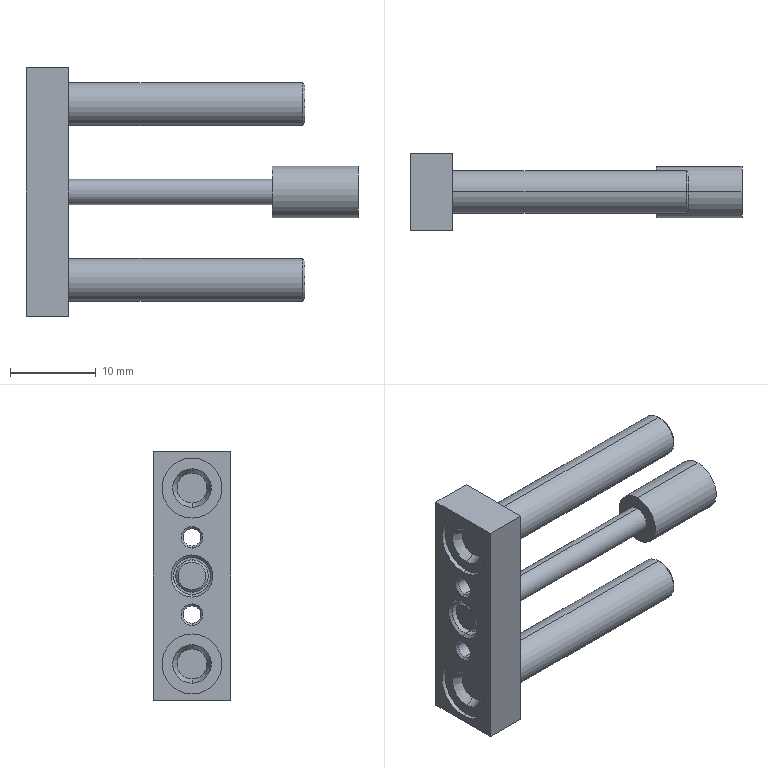Part | SolidWorks | features BaseBody 1 | 1 solid | 52 faces | box 38.7 x 9 x 29 mm | volume 2721 mm3 | cylinder 20 | cone 16 | plane 16 | commonest cylinder face diameters 2.013 x4 5 x4 7 x4 3 x2 3.8 x2 4.3 x2
STEP:
#1=CARTESIAN_POINT('',(0.2435,0.,-5.507));
#2=VERTEX_POINT('',#1);
#3=CARTESIAN_POINT('',(0.2435,0.,-3.494));
#4=VERTEX_POINT('',#3);
#5=CARTESIAN_POINT('',(0.2435,0.,-4.5));
#6=DIRECTION('',(1.,0.,0.));
#7=DIRECTION('',(0.,0.,1.));
#8=AXIS2_PLACEMENT_3D('',#5,#6,#7);
#9=CIRCLE('',#8,1.006);
#10=EDGE_CURVE('',#2,#4,#9,.T.);
#11=ORIENTED_EDGE('',*,*,#10,.F.);
#12=CARTESIAN_POINT('',(5.,0.,-5.507));
#13=VERTEX_POINT('',#12);
#14=CARTESIAN_POINT('',(5.,0.,-5.507));
#15=DIRECTION('',(1.,0.,0.));
#16=VECTOR('',#15,1000.);
#17=LINE('',#14,#16);
#18=EDGE_CURVE('',#2,#13,#17,.T.);
#19=ORIENTED_EDGE('',*,*,#18,.T.);
#20=CARTESIAN_POINT('',(5.,0.,-3.494));
#21=VERTEX_POINT('',#20);
#22=CARTESIAN_POINT('',(5.,0.,-4.5));
#23=DIRECTION('',(1.,0.,0.));
#24=DIRECTION('',(0.,0.,-1.));
#25=AXIS2_PLACEMENT_3D('',#22,#23,#24);
#26=CIRCLE('',#25,1.007);
#27=EDGE_CURVE('',#13,#21,#26,.T.);
#28=ORIENTED_EDGE('',*,*,#27,.T.);
#29=CARTESIAN_POINT('',(5.,0.,-3.494));
#30=DIRECTION('',(1.,0.,0.));
#31=VECTOR('',#30,1000.);
#32=LINE('',#29,#31);
#33=EDGE_CURVE('',#4,#21,#32,.T.);
#34=ORIENTED_EDGE('',*,*,#33,.F.);
#35=EDGE_LOOP('',(#11,#19,#28,#34));
#36=FACE_OUTER_BOUND('',#35,.T.);
#37=CARTESIAN_POINT('',(5.,0.,-4.5));
#38=DIRECTION('',(1.,0.,0.));
#39=DIRECTION('',(0.,0.,1.));
#40=AXIS2_PLACEMENT_3D('',#37,#38,#39);
#41=CYLINDRICAL_SURFACE('',#40,1.006);
#42=ADVANCED_FACE('',(#36),#41,.F.);
#43=ORIENTED_EDGE('',*,*,#10,.T.);
#44=CARTESIAN_POINT('',(0.,0.,-3.25));
#45=VERTEX_POINT('',#44);
#46=CARTESIAN_POINT('',(0.,0.,-3.25));
#47=DIRECTION('',(-0.7071,0.,0.7071));
#48=VECTOR('',#47,1000.);
#49=LINE('',#46,#48);
#50=EDGE_CURVE('',#4,#45,#49,.T.);
#51=ORIENTED_EDGE('',*,*,#50,.T.);
#52=CARTESIAN_POINT('',(0.,0.,-5.75));
#53=VERTEX_POINT('',#52);
#54=CARTESIAN_POINT('',(0.,0.,-4.5));
#55=DIRECTION('',(1.,0.,0.));
#56=DIRECTION('',(0.,-0.000000142,1.));
#57=AXIS2_PLACEMENT_3D('',#54,#55,#56);
#58=CIRCLE('',#57,1.25);
#59=EDGE_CURVE('',#53,#45,#58,.T.);
#60=ORIENTED_EDGE('',*,*,#59,.F.);
#61=CARTESIAN_POINT('',(0.,0.,-5.75));
#62=DIRECTION('',(-0.7071,0.,-0.7071));
#63=VECTOR('',#62,1000.);
#64=LINE('',#61,#63);
#65=EDGE_CURVE('',#2,#53,#64,.T.);
#66=ORIENTED_EDGE('',*,*,#65,.F.);
#67=EDGE_LOOP('',(#43,#51,#60,#66));
#68=FACE_OUTER_BOUND('',#67,.T.);
#69=CARTESIAN_POINT('',(0.,0.,-4.5));
#70=DIRECTION('',(-1.,0.,0.));
#71=DIRECTION('',(0.,0.,-1.));
#72=AXIS2_PLACEMENT_3D('',#69,#70,#71);
#73=CONICAL_SURFACE('',#72,1.25,0.7854);
#74=ADVANCED_FACE('',(#68),#73,.F.);
#75=CARTESIAN_POINT('',(0.2435,0.,3.494));
#76=VERTEX_POINT('',#75);
#77=CARTESIAN_POINT('',(0.2435,0.,5.507));
#78=VERTEX_POINT('',#77);
#79=CARTESIAN_POINT('',(0.2435,0.,4.5));
#80=DIRECTION('',(1.,0.,0.));
#81=DIRECTION('',(0.,0.,1.));
#82=AXIS2_PLACEMENT_3D('',#79,#80,#81);
#83=CIRCLE('',#82,1.007);
#84=EDGE_CURVE('',#76,#78,#83,.T.);
#85=ORIENTED_EDGE('',*,*,#84,.F.);
#86=CARTESIAN_POINT('',(5.,0.,3.494));
#87=VERTEX_POINT('',#86);
#88=CARTESIAN_POINT('',(5.,0.,3.494));
#89=DIRECTION('',(1.,0.,0.));
#90=VECTOR('',#89,1000.);
#91=LINE('',#88,#90);
#92=EDGE_CURVE('',#76,#87,#91,.T.);
#93=ORIENTED_EDGE('',*,*,#92,.T.);
#94=CARTESIAN_POINT('',(5.,0.,5.507));
#95=VERTEX_POINT('',#94);
#96=CARTESIAN_POINT('',(5.,0.,4.5));
#97=DIRECTION('',(1.,0.,0.));
#98=DIRECTION('',(0.,0.,-1.));
#99=AXIS2_PLACEMENT_3D('',#96,#97,#98);
#100=CIRCLE('',#99,1.006);
#101=EDGE_CURVE('',#87,#95,#100,.T.);
#102=ORIENTED_EDGE('',*,*,#101,.T.);
#103=CARTESIAN_POINT('',(5.,0.,5.507));
#104=DIRECTION('',(1.,0.,0.));
#105=VECTOR('',#104,1000.);
#106=LINE('',#103,#105);
#107=EDGE_CURVE('',#78,#95,#106,.T.);
#108=ORIENTED_EDGE('',*,*,#107,.F.);
#109=EDGE_LOOP('',(#85,#93,#102,#108));
#110=FACE_OUTER_BOUND('',#109,.T.);
#111=CARTESIAN_POINT('',(5.,0.,4.5));
#112=DIRECTION('',(1.,0.,0.));
#113=DIRECTION('',(0.,0.,1.));
#114=AXIS2_PLACEMENT_3D('',#111,#112,#113);
#115=CYLINDRICAL_SURFACE('',#114,1.007);
#116=ADVANCED_FACE('',(#110),#115,.F.);
#117=ORIENTED_EDGE('',*,*,#84,.T.);
#118=CARTESIAN_POINT('',(0.,0.,5.75));
#119=VERTEX_POINT('',#118);
#120=CARTESIAN_POINT('',(0.,0.,5.75));
#121=DIRECTION('',(-0.7071,0.,0.7071));
#122=VECTOR('',#121,1000.);
#123=LINE('',#120,#122);
#124=EDGE_CURVE('',#78,#119,#123,.T.);
#125=ORIENTED_EDGE('',*,*,#124,.T.);
#126=CARTESIAN_POINT('',(0.,0.,3.25));
#127=VERTEX_POINT('',#126);
#128=CARTESIAN_POINT('',(0.,0.,4.5));
#129=DIRECTION('',(1.,0.,0.));
#130=DIRECTION('',(0.,-0.000000142,1.));
#131=AXIS2_PLACEMENT_3D('',#128,#129,#130);
#132=CIRCLE('',#131,1.25);
#133=EDGE_CURVE('',#127,#119,#132,.T.);
#134=ORIENTED_EDGE('',*,*,#133,.F.);
#135=CARTESIAN_POINT('',(0.,0.,3.25));
#136=DIRECTION('',(-0.7071,0.,-0.7071));
#137=VECTOR('',#136,1000.);
#138=LINE('',#135,#137);
#139=EDGE_CURVE('',#76,#127,#138,.T.);
#140=ORIENTED_EDGE('',*,*,#139,.F.);
#141=EDGE_LOOP('',(#117,#125,#134,#140));
#142=FACE_OUTER_BOUND('',#141,.T.);
#143=CARTESIAN_POINT('',(0.,0.,4.5));
#144=DIRECTION('',(-1.,0.,0.));
#145=DIRECTION('',(0.,0.,-1.));
#146=AXIS2_PLACEMENT_3D('',#143,#144,#145);
#147=CONICAL_SURFACE('',#146,1.25,0.7854);
#148=ADVANCED_FACE('',(#142),#147,.F.);
#149=CARTESIAN_POINT('',(32.5,0.,-8.05));
#150=VERTEX_POINT('',#149);
#151=CARTESIAN_POINT('',(32.5,0.,-12.45));
#152=VERTEX_POINT('',#151);
#153=CARTESIAN_POINT('',(32.5,0.,-10.25));
#154=DIRECTION('',(1.,0.,0.));
#155=DIRECTION('',(0.,-0.000000143,1.));
#156=AXIS2_PLACEMENT_3D('',#153,#154,#155);
#157=CIRCLE('',#156,2.2);
#158=EDGE_CURVE('',#150,#152,#157,.T.);
#159=ORIENTED_EDGE('',*,*,#158,.F.);
#160=CARTESIAN_POINT('',(32.2,0.,-7.75));
#161=VERTEX_POINT('',#160);
#162=CARTESIAN_POINT('',(32.2,0.,-7.75));
#163=DIRECTION('',(-0.7071,0.,0.7071));
#164=VECTOR('',#163,1000.);
#165=LINE('',#162,#164);
#166=EDGE_CURVE('',#150,#161,#165,.T.);
#167=ORIENTED_EDGE('',*,*,#166,.T.);
#168=CARTESIAN_POINT('',(32.2,0.,-12.75));
#169=VERTEX_POINT('',#168);
#170=CARTESIAN_POINT('',(32.2,0.,-10.25));
#171=DIRECTION('',(1.,0.,0.));
#172=DIRECTION('',(0.,0.,-1.));
#173=AXIS2_PLACEMENT_3D('',#170,#171,#172);
#174=CIRCLE('',#173,2.5);
#175=EDGE_CURVE('',#161,#169,#174,.T.);
#176=ORIENTED_EDGE('',*,*,#175,.T.);
#177=CARTESIAN_POINT('',(32.2,0.,-12.75));
#178=DIRECTION('',(-0.7071,0.,-0.7071));
#179=VECTOR('',#178,1000.);
#180=LINE('',#177,#179);
#181=EDGE_CURVE('',#152,#169,#180,.T.);
#182=ORIENTED_EDGE('',*,*,#181,.F.);
#183=EDGE_LOOP('',(#159,#167,#176,#182));
#184=FACE_OUTER_BOUND('',#183,.T.);
#185=CARTESIAN_POINT('',(32.2,0.,-10.25));
#186=DIRECTION('',(-1.,0.,0.));
#187=DIRECTION('',(0.,0.,-1.));
#188=AXIS2_PLACEMENT_3D('',#185,#186,#187);
#189=CONICAL_SURFACE('',#188,2.5,0.7854);
#190=ADVANCED_FACE('',(#184),#189,.T.);
#191=CARTESIAN_POINT('',(5.,0.,-7.75));
#192=VERTEX_POINT('',#191);
#193=CARTESIAN_POINT('',(5.,0.,-12.75));
#194=VERTEX_POINT('',#193);
#195=CARTESIAN_POINT('',(5.,0.,-10.25));
#196=DIRECTION('',(1.,0.,0.));
#197=DIRECTION('',(0.,0.,-1.));
#198=AXIS2_PLACEMENT_3D('',#195,#196,#197);
#199=CIRCLE('',#198,2.5);
#200=EDGE_CURVE('',#192,#194,#199,.T.);
#201=ORIENTED_EDGE('',*,*,#200,.T.);
#202=CARTESIAN_POINT('',(32.5,0.,-12.75));
#203=DIRECTION('',(1.,0.,0.));
#204=VECTOR('',#203,1000.);
#205=LINE('',#202,#204);
#206=EDGE_CURVE('',#194,#169,#205,.T.);
#207=ORIENTED_EDGE('',*,*,#206,.T.);
#208=ORIENTED_EDGE('',*,*,#175,.F.);
#209=CARTESIAN_POINT('',(32.5,0.,-7.75));
#210=DIRECTION('',(1.,0.,0.));
#211=VECTOR('',#210,1000.);
#212=LINE('',#209,#211);
#213=EDGE_CURVE('',#192,#161,#212,.T.);
#214=ORIENTED_EDGE('',*,*,#213,.F.);
#215=EDGE_LOOP('',(#201,#207,#208,#214));
#216=FACE_OUTER_BOUND('',#215,.T.);
#217=CARTESIAN_POINT('',(32.5,0.,-10.25));
#218=DIRECTION('',(1.,0.,0.));
#219=DIRECTION('',(0.,0.,1.));
#220=AXIS2_PLACEMENT_3D('',#217,#218,#219);
#221=CYLINDRICAL_SURFACE('',#220,2.5);
#222=ADVANCED_FACE('',(#216),#221,.T.);
#223=CARTESIAN_POINT('',(32.5,0.,12.45));
#224=VERTEX_POINT('',#223);
#225=CARTESIAN_POINT('',(32.5,0.,8.05));
#226=VERTEX_POINT('',#225);
#227=CARTESIAN_POINT('',(32.5,0.,10.25));
#228=DIRECTION('',(1.,0.,0.));
#229=DIRECTION('',(0.,-0.000000143,1.));
#230=AXIS2_PLACEMENT_3D('',#227,#228,#229);
#231=CIRCLE('',#230,2.2);
#232=EDGE_CURVE('',#224,#226,#231,.T.);
#233=ORIENTED_EDGE('',*,*,#232,.F.);
#234=CARTESIAN_POINT('',(32.2,0.,12.75));
#235=VERTEX_POINT('',#234);
#236=CARTESIAN_POINT('',(32.2,0.,12.75));
#237=DIRECTION('',(-0.7071,0.,0.7071));
#238=VECTOR('',#237,1000.);
#239=LINE('',#236,#238);
#240=EDGE_CURVE('',#224,#235,#239,.T.);
#241=ORIENTED_EDGE('',*,*,#240,.T.);
#242=CARTESIAN_POINT('',(32.2,0.,7.75));
#243=VERTEX_POINT('',#242);
#244=CARTESIAN_POINT('',(32.2,0.,10.25));
#245=DIRECTION('',(1.,0.,0.));
#246=DIRECTION('',(0.,0.,-1.));
#247=AXIS2_PLACEMENT_3D('',#244,#245,#246);
#248=CIRCLE('',#247,2.5);
#249=EDGE_CURVE('',#235,#243,#248,.T.);
#250=ORIENTED_EDGE('',*,*,#249,.T.);
#251=CARTESIAN_POINT('',(32.2,0.,7.75));
#252=DIRECTION('',(-0.7071,0.,-0.7071));
#253=VECTOR('',#252,1000.);
#254=LINE('',#251,#253);
#255=EDGE_CURVE('',#226,#243,#254,.T.);
#256=ORIENTED_EDGE('',*,*,#255,.F.);
#257=EDGE_LOOP('',(#233,#241,#250,#256));
#258=FACE_OUTER_BOUND('',#257,.T.);
#259=CARTESIAN_POINT('',(32.2,0.,10.25));
#260=DIRECTION('',(-1.,0.,0.));
#261=DIRECTION('',(0.,0.,-1.));
#262=AXIS2_PLACEMENT_3D('',#259,#260,#261);
#263=CONICAL_SURFACE('',#262,2.5,0.7854);
#264=ADVANCED_FACE('',(#258),#263,.T.);
#265=CARTESIAN_POINT('',(5.,0.,12.75));
#266=VERTEX_POINT('',#265);
#267=CARTESIAN_POINT('',(5.,0.,7.75));
#268=VERTEX_POINT('',#267);
#269=CARTESIAN_POINT('',(5.,0.,10.25));
#270=DIRECTION('',(1.,0.,0.));
#271=DIRECTION('',(0.,0.,-1.));
#272=AXIS2_PLACEMENT_3D('',#269,#270,#271);
#273=CIRCLE('',#272,2.5);
#274=EDGE_CURVE('',#266,#268,#273,.T.);
#275=ORIENTED_EDGE('',*,*,#274,.T.);
#276=CARTESIAN_POINT('',(32.5,0.,7.75));
#277=DIRECTION('',(1.,0.,0.));
#278=VECTOR('',#277,1000.);
#279=LINE('',#276,#278);
#280=EDGE_CURVE('',#268,#243,#279,.T.);
#281=ORIENTED_EDGE('',*,*,#280,.T.);
#282=ORIENTED_EDGE('',*,*,#249,.F.);
#283=CARTESIAN_POINT('',(32.5,0.,12.75));
#284=DIRECTION('',(1.,0.,0.));
#285=VECTOR('',#284,1000.);
#286=LINE('',#283,#285);
#287=EDGE_CURVE('',#266,#235,#286,.T.);
#288=ORIENTED_EDGE('',*,*,#287,.F.);
#289=EDGE_LOOP('',(#275,#281,#282,#288));
#290=FACE_OUTER_BOUND('',#289,.T.);
#291=CARTESIAN_POINT('',(32.5,0.,10.25));
#292=DIRECTION('',(1.,0.,0.));
#293=DIRECTION('',(0.,0.,1.));
#294=AXIS2_PLACEMENT_3D('',#291,#292,#293);
#295=CYLINDRICAL_SURFACE('',#294,2.5);
#296=ADVANCED_FACE('',(#290),#295,.T.);
#297=CARTESIAN_POINT('',(0.5,0.,1.6));
#298=VERTEX_POINT('',#297);
#299=CARTESIAN_POINT('',(0.5,0.,-1.6));
#300=VERTEX_POINT('',#299);
#301=CARTESIAN_POINT('',(0.5,0.,0.));
#302=DIRECTION('',(1.,0.,0.));
#303=DIRECTION('',(0.,0.,-1.));
#304=AXIS2_PLACEMENT_3D('',#301,#302,#303);
#305=CIRCLE('',#304,1.6);
#306=EDGE_CURVE('',#298,#300,#305,.T.);
#307=ORIENTED_EDGE('',*,*,#306,.T.);
#308=CARTESIAN_POINT('',(0.8,0.,-1.9));
#309=VERTEX_POINT('',#308);
#310=CARTESIAN_POINT('',(0.8,0.,-1.9));
#311=DIRECTION('',(0.7071,0.,-0.7071));
#312=VECTOR('',#311,1000.);
#313=LINE('',#310,#312);
#314=EDGE_CURVE('',#300,#309,#313,.T.);
#315=ORIENTED_EDGE('',*,*,#314,.T.);
#316=CARTESIAN_POINT('',(0.8,0.,1.9));
#317=VERTEX_POINT('',#316);
#318=CARTESIAN_POINT('',(0.8,0.,0.));
#319=DIRECTION('',(1.,0.,0.));
#320=DIRECTION('',(0.,0.,1.));
#321=AXIS2_PLACEMENT_3D('',#318,#319,#320);
#322=CIRCLE('',#321,1.9);
#323=EDGE_CURVE('',#317,#309,#322,.T.);
#324=ORIENTED_EDGE('',*,*,#323,.F.);
#325=CARTESIAN_POINT('',(0.8,0.,1.9));
#326=DIRECTION('',(0.7071,0.,0.7071));
#327=VECTOR('',#326,1000.);
#328=LINE('',#325,#327);
#329=EDGE_CURVE('',#298,#317,#328,.T.);
#330=ORIENTED_EDGE('',*,*,#329,.F.);
#331=EDGE_LOOP('',(#307,#315,#324,#330));
#332=FACE_OUTER_BOUND('',#331,.T.);
#333=CARTESIAN_POINT('',(0.8,0.,0.));
#334=DIRECTION('',(1.,0.,0.));
#335=DIRECTION('',(0.,0.,1.));
#336=AXIS2_PLACEMENT_3D('',#333,#334,#335);
#337=CONICAL_SURFACE('',#336,1.9,0.7854);
#338=ADVANCED_FACE('',(#332),#337,.T.);
#339=ORIENTED_EDGE('',*,*,#323,.T.);
#340=CARTESIAN_POINT('',(2.5,0.,-1.9));
#341=VERTEX_POINT('',#340);
#342=CARTESIAN_POINT('',(2.5,0.,-1.9));
#343=DIRECTION('',(1.,0.,0.));
#344=VECTOR('',#343,1000.);
#345=LINE('',#342,#344);
#346=EDGE_CURVE('',#309,#341,#345,.T.);
#347=ORIENTED_EDGE('',*,*,#346,.T.);
#348=CARTESIAN_POINT('',(2.5,-0.000000271,1.9));
#349=VERTEX_POINT('',#348);
#350=CARTESIAN_POINT('',(2.5,0.,0.));
#351=DIRECTION('',(1.,0.,0.));
#352=DIRECTION('',(0.,-0.000000143,1.));
#353=AXIS2_PLACEMENT_3D('',#350,#351,#352);
#354=CIRCLE('',#353,1.9);
#355=EDGE_CURVE('',#349,#341,#354,.T.);
#356=ORIENTED_EDGE('',*,*,#355,.F.);
#357=CARTESIAN_POINT('',(2.5,0.,1.9));
#358=DIRECTION('',(1.,0.,0.));
#359=VECTOR('',#358,1000.);
#360=LINE('',#357,#359);
#361=EDGE_CURVE('',#317,#349,#360,.T.);
#362=ORIENTED_EDGE('',*,*,#361,.F.);
#363=EDGE_LOOP('',(#339,#347,#356,#362));
#364=FACE_OUTER_BOUND('',#363,.T.);
#365=CARTESIAN_POINT('',(2.5,0.,0.));
#366=DIRECTION('',(1.,0.,0.));
#367=DIRECTION('',(0.,0.,1.));
#368=AXIS2_PLACEMENT_3D('',#365,#366,#367);
#369=CYLINDRICAL_SURFACE('',#368,1.9);
#370=ADVANCED_FACE('',(#364),#369,.T.);
#371=CARTESIAN_POINT('',(0.3,0.,-2.15));
#372=VERTEX_POINT('',#371);
#373=CARTESIAN_POINT('',(0.3,0.,2.15));
#374=VERTEX_POINT('',#373);
#375=CARTESIAN_POINT('',(0.3,0.,0.));
#376=DIRECTION('',(1.,0.,0.));
#377=DIRECTION('',(0.,0.,1.));
#378=AXIS2_PLACEMENT_3D('',#375,#376,#377);
#379=CIRCLE('',#378,2.15);
#380=EDGE_CURVE('',#372,#374,#379,.T.);
#381=ORIENTED_EDGE('',*,*,#380,.F.);
#382=CARTESIAN_POINT('',(2.5,0.,-2.15));
#383=VERTEX_POINT('',#382);
#384=CARTESIAN_POINT('',(2.5,0.,-2.15));
#385=DIRECTION('',(1.,0.,0.));
#386=VECTOR('',#385,1000.);
#387=LINE('',#384,#386);
#388=EDGE_CURVE('',#372,#383,#387,.T.);
#389=ORIENTED_EDGE('',*,*,#388,.T.);
#390=CARTESIAN_POINT('',(2.5,0.,2.15));
#391=VERTEX_POINT('',#390);
#392=CARTESIAN_POINT('',(2.5,0.,0.));
#393=DIRECTION('',(1.,0.,0.));
#394=DIRECTION('',(0.,0.,-1.));
#395=AXIS2_PLACEMENT_3D('',#392,#393,#394);
#396=CIRCLE('',#395,2.15);
#397=EDGE_CURVE('',#383,#391,#396,.T.);
#398=ORIENTED_EDGE('',*,*,#397,.T.);
#399=CARTESIAN_POINT('',(2.5,0.,2.15));
#400=DIRECTION('',(1.,0.,0.));
#401=VECTOR('',#400,1000.);
#402=LINE('',#399,#401);
#403=EDGE_CURVE('',#374,#391,#402,.T.);
#404=ORIENTED_EDGE('',*,*,#403,.F.);
#405=EDGE_LOOP('',(#381,#389,#398,#404));
#406=FACE_OUTER_BOUND('',#405,.T.);
#407=CARTESIAN_POINT('',(2.5,0.,0.));
#408=DIRECTION('',(1.,0.,0.));
#409=DIRECTION('',(0.,0.,1.));
#410=AXIS2_PLACEMENT_3D('',#407,#408,#409);
#411=CYLINDRICAL_SURFACE('',#410,2.15);
#412=ADVANCED_FACE('',(#406),#411,.F.);
#413=ORIENTED_EDGE('',*,*,#380,.T.);
#414=CARTESIAN_POINT('',(0.,0.,2.45));
#415=VERTEX_POINT('',#414);
#416=CARTESIAN_POINT('',(0.,0.,2.45));
#417=DIRECTION('',(-0.7071,0.,0.7071));
#418=VECTOR('',#417,1000.);
#419=LINE('',#416,#418);
#420=EDGE_CURVE('',#374,#415,#419,.T.);
#421=ORIENTED_EDGE('',*,*,#420,.T.);
#422=CARTESIAN_POINT('',(0.,0.,-2.45));
#423=VERTEX_POINT('',#422);
#424=CARTESIAN_POINT('',(0.,0.,0.));
#425=DIRECTION('',(1.,0.,0.));
#426=DIRECTION('',(0.,-0.000000142,1.));
#427=AXIS2_PLACEMENT_3D('',#424,#425,#426);
#428=CIRCLE('',#427,2.45);
#429=EDGE_CURVE('',#423,#415,#428,.T.);
#430=ORIENTED_EDGE('',*,*,#429,.F.);
#431=CARTESIAN_POINT('',(0.,0.,-2.45));
#432=DIRECTION('',(-0.7071,0.,-0.7071));
#433=VECTOR('',#432,1000.);
#434=LINE('',#431,#433);
#435=EDGE_CURVE('',#372,#423,#434,.T.);
#436=ORIENTED_EDGE('',*,*,#435,.F.);
#437=EDGE_LOOP('',(#413,#421,#430,#436));
#438=FACE_OUTER_BOUND('',#437,.T.);
#439=CARTESIAN_POINT('',(0.,0.,0.));
#440=DIRECTION('',(-1.,0.,0.));
#441=DIRECTION('',(0.,0.,-1.));
#442=AXIS2_PLACEMENT_3D('',#439,#440,#441);
#443=CONICAL_SURFACE('',#442,2.45,0.7854);
#444=ADVANCED_FACE('',(#438),#443,.F.);
#445=CARTESIAN_POINT('',(1.6,0.,-12.));
#446=VERTEX_POINT('',#445);
#447=CARTESIAN_POINT('',(1.6,0.,-8.5));
#448=VERTEX_POINT('',#447);
#449=CARTESIAN_POINT('',(1.6,0.,-10.25));
#450=DIRECTION('',(1.,0.,0.));
#451=DIRECTION('',(0.,0.,-1.));
#452=AXIS2_PLACEMENT_3D('',#449,#450,#451);
#453=CIRCLE('',#452,1.75);
#454=EDGE_CURVE('',#446,#448,#453,.T.);
#455=ORIENTED_EDGE('',*,*,#454,.T.);
#456=CARTESIAN_POINT('',(0.5,0.,-8.));
#457=VERTEX_POINT('',#456);
#458=CARTESIAN_POINT('',(0.5,0.,-8.));
#459=DIRECTION('',(-0.9104,0.,0.4138));
#460=VECTOR('',#459,1000.);
#461=LINE('',#458,#460);
#462=EDGE_CURVE('',#448,#457,#461,.T.);
#463=ORIENTED_EDGE('',*,*,#462,.T.);
#464=CARTESIAN_POINT('',(0.5,0.,-12.5));
#465=VERTEX_POINT('',#464);
#466=CARTESIAN_POINT('',(0.5,0.,-10.25));
#467=DIRECTION('',(1.,0.,0.));
#468=DIRECTION('',(0.,-0.000000142,1.));
#469=AXIS2_PLACEMENT_3D('',#466,#467,#468);
#470=CIRCLE('',#469,2.25);
#471=EDGE_CURVE('',#465,#457,#470,.T.);
#472=ORIENTED_EDGE('',*,*,#471,.F.);
#473=CARTESIAN_POINT('',(0.5,0.,-12.5));
#474=DIRECTION('',(-0.9104,0.,-0.4138));
#475=VECTOR('',#474,1000.);
#476=LINE('',#473,#475);
#477=EDGE_CURVE('',#446,#465,#476,.T.);
#478=ORIENTED_EDGE('',*,*,#477,.F.);
#479=EDGE_LOOP('',(#455,#463,#472,#478));
#480=FACE_OUTER_BOUND('',#479,.T.);
#481=CARTESIAN_POINT('',(0.5,0.,-10.25));
#482=DIRECTION('',(-1.,0.,0.));
#483=DIRECTION('',(0.,0.,-1.));
#484=AXIS2_PLACEMENT_3D('',#481,#482,#483);
#485=CONICAL_SURFACE('',#484,2.25,0.4266);
#486=ADVANCED_FACE('',(#480),#485,.F.);
#487=CARTESIAN_POINT('',(0.,-0.000000497,-13.75));
#488=VERTEX_POINT('',#487);
#489=CARTESIAN_POINT('',(0.,0.,-6.75));
#490=VERTEX_POINT('',#489);
#491=CARTESIAN_POINT('',(0.,0.,-10.25));
#492=DIRECTION('',(1.,0.,0.));
#493=DIRECTION('',(0.,0.,1.));
#494=AXIS2_PLACEMENT_3D('',#491,#492,#493);
#495=CIRCLE('',#494,3.5);
#496=EDGE_CURVE('',#488,#490,#495,.T.);
#497=ORIENTED_EDGE('',*,*,#496,.F.);
#498=CARTESIAN_POINT('',(0.5,-0.000000497,-13.75));
#499=VERTEX_POINT('',#498);
#500=CARTESIAN_POINT('',(1.6,-0.000000497,-13.75));
#501=DIRECTION('',(1.,0.,0.));
#502=VECTOR('',#501,1000.);
#503=LINE('',#500,#502);
#504=EDGE_CURVE('',#488,#499,#503,.T.);
#505=ORIENTED_EDGE('',*,*,#504,.T.);
#506=CARTESIAN_POINT('',(0.5,0.000000497,-6.75));
#507=VERTEX_POINT('',#506);
#508=CARTESIAN_POINT('',(0.5,0.,-10.25));
#509=DIRECTION('',(1.,0.,0.));
#510=DIRECTION('',(0.,0.,-1.));
#511=AXIS2_PLACEMENT_3D('',#508,#509,#510);
#512=CIRCLE('',#511,3.5);
#513=EDGE_CURVE('',#499,#507,#512,.T.);
#514=ORIENTED_EDGE('',*,*,#513,.T.);
#515=CARTESIAN_POINT('',(1.6,0.000000497,-6.75));
#516=DIRECTION('',(1.,0.,0.));
#517=VECTOR('',#516,1000.);
#518=LINE('',#515,#517);
#519=EDGE_CURVE('',#490,#507,#518,.T.);
#520=ORIENTED_EDGE('',*,*,#519,.F.);
#521=EDGE_LOOP('',(#497,#505,#514,#520));
#522=FACE_OUTER_BOUND('',#521,.T.);
#523=CARTESIAN_POINT('',(1.6,0.,-10.25));
#524=DIRECTION('',(1.,0.,0.));
#525=DIRECTION('',(0.,0.000000142,1.));
#526=AXIS2_PLACEMENT_3D('',#523,#524,#525);
#527=CYLINDRICAL_SURFACE('',#526,3.5);
#528=ADVANCED_FACE('',(#522),#527,.F.);
#529=CARTESIAN_POINT('',(1.6,0.,8.5));
#530=VERTEX_POINT('',#529);
#531=CARTESIAN_POINT('',(1.6,0.,12.));
#532=VERTEX_POINT('',#531);
#533=CARTESIAN_POINT('',(1.6,0.,10.25));
#534=DIRECTION('',(1.,0.,0.));
#535=DIRECTION('',(0.,0.,-1.));
#536=AXIS2_PLACEMENT_3D('',#533,#534,#535);
#537=CIRCLE('',#536,1.75);
#538=EDGE_CURVE('',#530,#532,#537,.T.);
#539=ORIENTED_EDGE('',*,*,#538,.T.);
#540=CARTESIAN_POINT('',(0.5,0.,12.5));
#541=VERTEX_POINT('',#540);
#542=CARTESIAN_POINT('',(0.5,0.,12.5));
#543=DIRECTION('',(-0.9104,0.,0.4138));
#544=VECTOR('',#543,1000.);
#545=LINE('',#542,#544);
#546=EDGE_CURVE('',#532,#541,#545,.T.);
#547=ORIENTED_EDGE('',*,*,#546,.T.);
#548=CARTESIAN_POINT('',(0.5,0.,8.));
#549=VERTEX_POINT('',#548);
#550=CARTESIAN_POINT('',(0.5,0.,10.25));
#551=DIRECTION('',(1.,0.,0.));
#552=DIRECTION('',(0.,-0.000000142,1.));
#553=AXIS2_PLACEMENT_3D('',#550,#551,#552);
#554=CIRCLE('',#553,2.25);
#555=EDGE_CURVE('',#549,#541,#554,.T.);
#556=ORIENTED_EDGE('',*,*,#555,.F.);
#557=CARTESIAN_POINT('',(0.5,0.,8.));
#558=DIRECTION('',(-0.9104,0.,-0.4138));
#559=VECTOR('',#558,1000.);
#560=LINE('',#557,#559);
#561=EDGE_CURVE('',#530,#549,#560,.T.);
#562=ORIENTED_EDGE('',*,*,#561,.F.);
#563=EDGE_LOOP('',(#539,#547,#556,#562));
#564=FACE_OUTER_BOUND('',#563,.T.);
#565=CARTESIAN_POINT('',(0.5,0.,10.25));
#566=DIRECTION('',(-1.,0.,0.));
#567=DIRECTION('',(0.,0.,-1.));
#568=AXIS2_PLACEMENT_3D('',#565,#566,#567);
#569=CONICAL_SURFACE('',#568,2.25,0.4266);
#570=ADVANCED_FACE('',(#564),#569,.F.);
#571=CARTESIAN_POINT('',(0.,-0.000000498,6.75));
#572=VERTEX_POINT('',#571);
#573=CARTESIAN_POINT('',(0.,0.,13.75));
#574=VERTEX_POINT('',#573);
#575=CARTESIAN_POINT('',(0.,0.,10.25));
#576=DIRECTION('',(1.,0.,0.));
#577=DIRECTION('',(0.,0.,1.));
#578=AXIS2_PLACEMENT_3D('',#575,#576,#577);
#579=CIRCLE('',#578,3.5);
#580=EDGE_CURVE('',#572,#574,#579,.T.);
#581=ORIENTED_EDGE('',*,*,#580,.F.);
#582=CARTESIAN_POINT('',(0.5,-0.000000498,6.75));
#583=VERTEX_POINT('',#582);
#584=CARTESIAN_POINT('',(1.6,-0.000000498,6.75));
#585=DIRECTION('',(1.,0.,0.));
#586=VECTOR('',#585,1000.);
#587=LINE('',#584,#586);
#588=EDGE_CURVE('',#572,#583,#587,.T.);
#589=ORIENTED_EDGE('',*,*,#588,.T.);
#590=CARTESIAN_POINT('',(0.5,0.000000498,13.75));
#591=VERTEX_POINT('',#590);
#592=CARTESIAN_POINT('',(0.5,0.,10.25));
#593=DIRECTION('',(1.,0.,0.));
#594=DIRECTION('',(0.,0.,-1.));
#595=AXIS2_PLACEMENT_3D('',#592,#593,#594);
#596=CIRCLE('',#595,3.5);
#597=EDGE_CURVE('',#583,#591,#596,.T.);
#598=ORIENTED_EDGE('',*,*,#597,.T.);
#599=CARTESIAN_POINT('',(1.6,0.000000498,13.75));
#600=DIRECTION('',(1.,0.,0.));
#601=VECTOR('',#600,1000.);
#602=LINE('',#599,#601);
#603=EDGE_CURVE('',#574,#591,#602,.T.);
#604=ORIENTED_EDGE('',*,*,#603,.F.);
#605=EDGE_LOOP('',(#581,#589,#598,#604));
#606=FACE_OUTER_BOUND('',#605,.T.);
#607=CARTESIAN_POINT('',(1.6,0.,10.25));
#608=DIRECTION('',(1.,0.,0.));
#609=DIRECTION('',(0.,0.000000142,1.));
#610=AXIS2_PLACEMENT_3D('',#607,#608,#609);
#611=CYLINDRICAL_SURFACE('',#610,3.5);
#612=ADVANCED_FACE('',(#606),#611,.F.);
#613=CARTESIAN_POINT('',(28.7,0.,3.));
#614=VERTEX_POINT('',#613);
#615=CARTESIAN_POINT('',(28.7,0.,-3.));
#616=VERTEX_POINT('',#615);
#617=CARTESIAN_POINT('',(28.7,0.,0.));
#618=DIRECTION('',(1.,0.,0.));
#619=DIRECTION('',(0.,0.,-1.));
#620=AXIS2_PLACEMENT_3D('',#617,#618,#619);
#621=CIRCLE('',#620,3.);
#622=EDGE_CURVE('',#614,#616,#621,.T.);
#623=ORIENTED_EDGE('',*,*,#622,.T.);
#624=CARTESIAN_POINT('',(38.7,0.,-3.));
#625=VERTEX_POINT('',#624);
#626=CARTESIAN_POINT('',(38.7,0.,-3.));
#627=DIRECTION('',(1.,0.,0.));
#628=VECTOR('',#627,1000.);
#629=LINE('',#626,#628);
#630=EDGE_CURVE('',#616,#625,#629,.T.);
#631=ORIENTED_EDGE('',*,*,#630,.T.);
#632=CARTESIAN_POINT('',(38.7,0.,3.));
#633=VERTEX_POINT('',#632);
#634=CARTESIAN_POINT('',(38.7,0.,0.));
#635=DIRECTION('',(1.,0.,0.));
#636=DIRECTION('',(0.,0.,1.));
#637=AXIS2_PLACEMENT_3D('',#634,#635,#636);
#638=CIRCLE('',#637,3.);
#639=EDGE_CURVE('',#633,#625,#638,.T.);
#640=ORIENTED_EDGE('',*,*,#639,.F.);
#641=CARTESIAN_POINT('',(38.7,0.,3.));
#642=DIRECTION('',(1.,0.,0.));
#643=VECTOR('',#642,1000.);
#644=LINE('',#641,#643);
#645=EDGE_CURVE('',#614,#633,#644,.T.);
#646=ORIENTED_EDGE('',*,*,#645,.F.);
#647=EDGE_LOOP('',(#623,#631,#640,#646));
#648=FACE_OUTER_BOUND('',#647,.T.);
#649=CARTESIAN_POINT('',(38.7,0.,0.));
#650=DIRECTION('',(1.,0.,0.));
#651=DIRECTION('',(0.,0.,1.));
#652=AXIS2_PLACEMENT_3D('',#649,#650,#651);
#653=CYLINDRICAL_SURFACE('',#652,3.);
#654=ADVANCED_FACE('',(#648),#653,.T.);
#655=CARTESIAN_POINT('',(5.,0.,1.5));
#656=VERTEX_POINT('',#655);
#657=CARTESIAN_POINT('',(5.,0.,-1.5));
#658=VERTEX_POINT('',#657);
#659=CARTESIAN_POINT('',(5.,0.,0.));
#660=DIRECTION('',(1.,0.,0.));
#661=DIRECTION('',(0.,0.,-1.));
#662=AXIS2_PLACEMENT_3D('',#659,#660,#661);
#663=CIRCLE('',#662,1.5);
#664=EDGE_CURVE('',#656,#658,#663,.T.);
#665=ORIENTED_EDGE('',*,*,#664,.T.);
#666=CARTESIAN_POINT('',(28.7,0.,-1.5));
#667=VERTEX_POINT('',#666);
#668=CARTESIAN_POINT('',(38.7,0.,-1.5));
#669=DIRECTION('',(1.,0.,0.));
#670=VECTOR('',#669,1000.);
#671=LINE('',#668,#670);
#672=EDGE_CURVE('',#658,#667,#671,.T.);
#673=ORIENTED_EDGE('',*,*,#672,.T.);
#674=CARTESIAN_POINT('',(28.7,0.,1.5));
#675=VERTEX_POINT('',#674);
#676=CARTESIAN_POINT('',(28.7,0.,0.));
#677=DIRECTION('',(1.,0.,0.));
#678=DIRECTION('',(0.,0.,1.));
#679=AXIS2_PLACEMENT_3D('',#676,#677,#678);
#680=CIRCLE('',#679,1.5);
#681=EDGE_CURVE('',#675,#667,#680,.T.);
#682=ORIENTED_EDGE('',*,*,#681,.F.);
#683=CARTESIAN_POINT('',(38.7,0.,1.5));
#684=DIRECTION('',(1.,0.,0.));
#685=VECTOR('',#684,1000.);
#686=LINE('',#683,#685);
#687=EDGE_CURVE('',#656,#675,#686,.T.);
#688=ORIENTED_EDGE('',*,*,#687,.F.);
#689=EDGE_LOOP('',(#665,#673,#682,#688));
#690=FACE_OUTER_BOUND('',#689,.T.);
#691=CARTESIAN_POINT('',(38.7,0.,0.));
#692=DIRECTION('',(1.,0.,0.));
#693=DIRECTION('',(0.,0.,1.));
#694=AXIS2_PLACEMENT_3D('',#691,#692,#693);
#695=CYLINDRICAL_SURFACE('',#694,1.5);
#696=ADVANCED_FACE('',(#690),#695,.T.);
#697=CARTESIAN_POINT('',(0.,4.5,-14.5));
#698=VERTEX_POINT('',#697);
#699=CARTESIAN_POINT('',(0.,4.5,14.5));
#700=VERTEX_POINT('',#699);
#701=CARTESIAN_POINT('',(0.,4.5,-14.5));
#702=DIRECTION('',(0.,0.,1.));
#703=VECTOR('',#702,1000.);
#704=LINE('',#701,#703);
#705=EDGE_CURVE('',#698,#700,#704,.T.);
#706=ORIENTED_EDGE('',*,*,#705,.T.);
#707=CARTESIAN_POINT('',(5.,4.5,14.5));
#708=VERTEX_POINT('',#707);
#709=CARTESIAN_POINT('',(0.,4.5,14.5));
#710=DIRECTION('',(-1.,0.,0.));
#711=VECTOR('',#710,1000.);
#712=LINE('',#709,#711);
#713=EDGE_CURVE('',#708,#700,#712,.T.);
#714=ORIENTED_EDGE('',*,*,#713,.F.);
#715=CARTESIAN_POINT('',(5.,4.5,-14.5));
#716=VERTEX_POINT('',#715);
#717=CARTESIAN_POINT('',(5.,4.5,14.5));
#718=DIRECTION('',(0.,0.,1.));
#719=VECTOR('',#718,1000.);
#720=LINE('',#717,#719);
#721=EDGE_CURVE('',#716,#708,#720,.T.);
#722=ORIENTED_EDGE('',*,*,#721,.F.);
#723=CARTESIAN_POINT('',(5.,4.5,-14.5));
#724=DIRECTION('',(-1.,0.,0.));
#725=VECTOR('',#724,1000.);
#726=LINE('',#723,#725);
#727=EDGE_CURVE('',#716,#698,#726,.T.);
#728=ORIENTED_EDGE('',*,*,#727,.T.);
#729=EDGE_LOOP('',(#706,#714,#722,#728));
#730=FACE_OUTER_BOUND('',#729,.T.);
#731=CARTESIAN_POINT('',(0.,4.5,14.5));
#732=DIRECTION('',(0.,1.,0.));
#733=DIRECTION('',(1.,0.,0.));
#734=AXIS2_PLACEMENT_3D('',#731,#732,#733);
#735=PLANE('',#734);
#736=ADVANCED_FACE('',(#730),#735,.T.);
#737=CARTESIAN_POINT('',(0.,-4.5,14.5));
#738=VERTEX_POINT('',#737);
#739=CARTESIAN_POINT('',(0.,4.5,14.5));
#740=DIRECTION('',(0.,-1.,0.));
#741=VECTOR('',#740,1000.);
#742=LINE('',#739,#741);
#743=EDGE_CURVE('',#700,#738,#742,.T.);
#744=ORIENTED_EDGE('',*,*,#743,.T.);
#745=CARTESIAN_POINT('',(5.,-4.5,14.5));
#746=VERTEX_POINT('',#745);
#747=CARTESIAN_POINT('',(0.,-4.5,14.5));
#748=DIRECTION('',(-1.,0.,0.));
#749=VECTOR('',#748,1000.);
#750=LINE('',#747,#749);
#751=EDGE_CURVE('',#746,#738,#750,.T.);
#752=ORIENTED_EDGE('',*,*,#751,.F.);
#753=CARTESIAN_POINT('',(5.,-4.5,14.5));
#754=DIRECTION('',(0.,-1.,0.));
#755=VECTOR('',#754,1000.);
#756=LINE('',#753,#755);
#757=EDGE_CURVE('',#708,#746,#756,.T.);
#758=ORIENTED_EDGE('',*,*,#757,.F.);
#759=ORIENTED_EDGE('',*,*,#713,.T.);
#760=EDGE_LOOP('',(#744,#752,#758,#759));
#761=FACE_OUTER_BOUND('',#760,.T.);
#762=CARTESIAN_POINT('',(5.,-4.5,14.5));
#763=DIRECTION('',(0.,0.,1.));
#764=DIRECTION('',(0.,1.,0.));
#765=AXIS2_PLACEMENT_3D('',#762,#763,#764);
#766=PLANE('',#765);
#767=ADVANCED_FACE('',(#761),#766,.T.);
#768=CARTESIAN_POINT('',(0.,-4.5,-14.5));
#769=VERTEX_POINT('',#768);
#770=CARTESIAN_POINT('',(0.,-4.5,14.5));
#771=DIRECTION('',(0.,0.,-1.));
#772=VECTOR('',#771,1000.);
#773=LINE('',#770,#772);
#774=EDGE_CURVE('',#738,#769,#773,.T.);
#775=ORIENTED_EDGE('',*,*,#774,.T.);
#776=CARTESIAN_POINT('',(5.,-4.5,-14.5));
#777=VERTEX_POINT('',#776);
#778=CARTESIAN_POINT('',(0.,-4.5,-14.5));
#779=DIRECTION('',(-1.,0.,0.));
#780=VECTOR('',#779,1000.);
#781=LINE('',#778,#780);
#782=EDGE_CURVE('',#777,#769,#781,.T.);
#783=ORIENTED_EDGE('',*,*,#782,.F.);
#784=CARTESIAN_POINT('',(5.,-4.5,-14.5));
#785=DIRECTION('',(0.,0.,-1.));
#786=VECTOR('',#785,1000.);
#787=LINE('',#784,#786);
#788=EDGE_CURVE('',#746,#777,#787,.T.);
#789=ORIENTED_EDGE('',*,*,#788,.F.);
#790=ORIENTED_EDGE('',*,*,#751,.T.);
#791=EDGE_LOOP('',(#775,#783,#789,#790));
#792=FACE_OUTER_BOUND('',#791,.T.);
#793=CARTESIAN_POINT('',(0.,-4.5,-14.5));
#794=DIRECTION('',(0.,-1.,0.));
#795=DIRECTION('',(1.,0.,0.));
#796=AXIS2_PLACEMENT_3D('',#793,#794,#795);
#797=PLANE('',#796);
#798=ADVANCED_FACE('',(#792),#797,.T.);
#799=CARTESIAN_POINT('',(0.,-4.5,-14.5));
#800=DIRECTION('',(0.,1.,0.));
#801=VECTOR('',#800,1000.);
#802=LINE('',#799,#801);
#803=EDGE_CURVE('',#769,#698,#802,.T.);
#804=ORIENTED_EDGE('',*,*,#803,.T.);
#805=ORIENTED_EDGE('',*,*,#727,.F.);
#806=CARTESIAN_POINT('',(5.,4.5,-14.5));
#807=DIRECTION('',(0.,1.,0.));
#808=VECTOR('',#807,1000.);
#809=LINE('',#806,#808);
#810=EDGE_CURVE('',#777,#716,#809,.T.);
#811=ORIENTED_EDGE('',*,*,#810,.F.);
#812=ORIENTED_EDGE('',*,*,#782,.T.);
#813=EDGE_LOOP('',(#804,#805,#811,#812));
#814=FACE_OUTER_BOUND('',#813,.T.);
#815=CARTESIAN_POINT('',(0.,-4.5,-14.5));
#816=DIRECTION('',(0.,0.,-1.));
#817=DIRECTION('',(0.,1.,0.));
#818=AXIS2_PLACEMENT_3D('',#815,#816,#817);
#819=PLANE('',#818);
#820=ADVANCED_FACE('',(#814),#819,.T.);
#821=ORIENTED_EDGE('',*,*,#721,.T.);
#822=ORIENTED_EDGE('',*,*,#757,.T.);
#823=ORIENTED_EDGE('',*,*,#788,.T.);
#824=ORIENTED_EDGE('',*,*,#810,.T.);
#825=EDGE_LOOP('',(#821,#822,#823,#824));
#826=FACE_OUTER_BOUND('',#825,.T.);
#827=ORIENTED_EDGE('',*,*,#274,.F.);
#828=CARTESIAN_POINT('',(5.,0.,10.25));
#829=DIRECTION('',(1.,0.,0.));
#830=DIRECTION('',(0.,0.,-1.));
#831=AXIS2_PLACEMENT_3D('',#828,#829,#830);
#832=CIRCLE('',#831,2.5);
#833=EDGE_CURVE('',#268,#266,#832,.T.);
#834=ORIENTED_EDGE('',*,*,#833,.F.);
#835=EDGE_LOOP('',(#827,#834));
#836=FACE_BOUND('',#835,.T.);
#837=ORIENTED_EDGE('',*,*,#200,.F.);
#838=CARTESIAN_POINT('',(5.,0.,-10.25));
#839=DIRECTION('',(1.,0.,0.));
#840=DIRECTION('',(0.,0.,-1.));
#841=AXIS2_PLACEMENT_3D('',#838,#839,#840);
#842=CIRCLE('',#841,2.5);
#843=EDGE_CURVE('',#194,#192,#842,.T.);
#844=ORIENTED_EDGE('',*,*,#843,.F.);
#845=EDGE_LOOP('',(#837,#844));
#846=FACE_BOUND('',#845,.T.);
#847=ORIENTED_EDGE('',*,*,#664,.F.);
#848=CARTESIAN_POINT('',(5.,0.,0.));
#849=DIRECTION('',(1.,0.,0.));
#850=DIRECTION('',(0.,0.,-1.));
#851=AXIS2_PLACEMENT_3D('',#848,#849,#850);
#852=CIRCLE('',#851,1.5);
#853=EDGE_CURVE('',#658,#656,#852,.T.);
#854=ORIENTED_EDGE('',*,*,#853,.F.);
#855=EDGE_LOOP('',(#847,#854));
#856=FACE_BOUND('',#855,.T.);
#857=CARTESIAN_POINT('',(5.,0.,-4.5));
#858=DIRECTION('',(1.,0.,0.));
#859=DIRECTION('',(0.,0.,-1.));
#860=AXIS2_PLACEMENT_3D('',#857,#858,#859);
#861=CIRCLE('',#860,1.007);
#862=EDGE_CURVE('',#21,#13,#861,.T.);
#863=ORIENTED_EDGE('',*,*,#862,.F.);
#864=ORIENTED_EDGE('',*,*,#27,.F.);
#865=EDGE_LOOP('',(#863,#864));
#866=FACE_BOUND('',#865,.T.);
#867=CARTESIAN_POINT('',(5.,0.,4.5));
#868=DIRECTION('',(1.,0.,0.));
#869=DIRECTION('',(0.,0.,-1.));
#870=AXIS2_PLACEMENT_3D('',#867,#868,#869);
#871=CIRCLE('',#870,1.006);
#872=EDGE_CURVE('',#95,#87,#871,.T.);
#873=ORIENTED_EDGE('',*,*,#872,.F.);
#874=ORIENTED_EDGE('',*,*,#101,.F.);
#875=EDGE_LOOP('',(#873,#874));
#876=FACE_BOUND('',#875,.T.);
#877=CARTESIAN_POINT('',(5.,-4.5,14.5));
#878=DIRECTION('',(1.,0.,0.));
#879=DIRECTION('',(0.,0.,-1.));
#880=AXIS2_PLACEMENT_3D('',#877,#878,#879);
#881=PLANE('',#880);
#882=ADVANCED_FACE('',(#826,#836,#846,#856,#866,#876),#881,.T.);
#883=ORIENTED_EDGE('',*,*,#705,.F.);
#884=ORIENTED_EDGE('',*,*,#803,.F.);
#885=ORIENTED_EDGE('',*,*,#774,.F.);
#886=ORIENTED_EDGE('',*,*,#743,.F.);
#887=EDGE_LOOP('',(#883,#884,#885,#886));
#888=FACE_OUTER_BOUND('',#887,.T.);
#889=CARTESIAN_POINT('',(0.,0.,10.25));
#890=DIRECTION('',(1.,0.,0.));
#891=DIRECTION('',(0.,0.,1.));
#892=AXIS2_PLACEMENT_3D('',#889,#890,#891);
#893=CIRCLE('',#892,3.5);
#894=EDGE_CURVE('',#574,#572,#893,.T.);
#895=ORIENTED_EDGE('',*,*,#894,.T.);
#896=ORIENTED_EDGE('',*,*,#580,.T.);
#897=EDGE_LOOP('',(#895,#896));
#898=FACE_BOUND('',#897,.T.);
#899=CARTESIAN_POINT('',(0.,0.,-10.25));
#900=DIRECTION('',(1.,0.,0.));
#901=DIRECTION('',(0.,0.,1.));
#902=AXIS2_PLACEMENT_3D('',#899,#900,#901);
#903=CIRCLE('',#902,3.5);
#904=EDGE_CURVE('',#490,#488,#903,.T.);
#905=ORIENTED_EDGE('',*,*,#904,.T.);
#906=ORIENTED_EDGE('',*,*,#496,.T.);
#907=EDGE_LOOP('',(#905,#906));
#908=FACE_BOUND('',#907,.T.);
#909=ORIENTED_EDGE('',*,*,#429,.T.);
#910=CARTESIAN_POINT('',(0.,0.,0.));
#911=DIRECTION('',(1.,0.,0.));
#912=DIRECTION('',(0.,-0.000000142,1.));
#913=AXIS2_PLACEMENT_3D('',#910,#911,#912);
#914=CIRCLE('',#913,2.45);
#915=EDGE_CURVE('',#415,#423,#914,.T.);
#916=ORIENTED_EDGE('',*,*,#915,.T.);
#917=EDGE_LOOP('',(#909,#916));
#918=FACE_BOUND('',#917,.T.);
#919=ORIENTED_EDGE('',*,*,#59,.T.);
#920=CARTESIAN_POINT('',(0.,0.,-4.5));
#921=DIRECTION('',(1.,0.,0.));
#922=DIRECTION('',(0.,-0.000000142,1.));
#923=AXIS2_PLACEMENT_3D('',#920,#921,#922);
#924=CIRCLE('',#923,1.25);
#925=EDGE_CURVE('',#45,#53,#924,.T.);
#926=ORIENTED_EDGE('',*,*,#925,.T.);
#927=EDGE_LOOP('',(#919,#926));
#928=FACE_BOUND('',#927,.T.);
#929=ORIENTED_EDGE('',*,*,#133,.T.);
#930=CARTESIAN_POINT('',(0.,0.,4.5));
#931=DIRECTION('',(1.,0.,0.));
#932=DIRECTION('',(0.,-0.000000142,1.));
#933=AXIS2_PLACEMENT_3D('',#930,#931,#932);
#934=CIRCLE('',#933,1.25);
#935=EDGE_CURVE('',#119,#127,#934,.T.);
#936=ORIENTED_EDGE('',*,*,#935,.T.);
#937=EDGE_LOOP('',(#929,#936));
#938=FACE_BOUND('',#937,.T.);
#939=CARTESIAN_POINT('',(0.,-4.5,14.5));
#940=DIRECTION('',(-1.,0.,0.));
#941=DIRECTION('',(0.,1.,0.));
#942=AXIS2_PLACEMENT_3D('',#939,#940,#941);
#943=PLANE('',#942);
#944=ADVANCED_FACE('',(#888,#898,#908,#918,#928,#938),#943,.T.);
#945=ORIENTED_EDGE('',*,*,#622,.F.);
#946=CARTESIAN_POINT('',(28.7,0.,0.));
#947=DIRECTION('',(1.,0.,0.));
#948=DIRECTION('',(0.,0.,-1.));
#949=AXIS2_PLACEMENT_3D('',#946,#947,#948);
#950=CIRCLE('',#949,3.);
#951=EDGE_CURVE('',#616,#614,#950,.T.);
#952=ORIENTED_EDGE('',*,*,#951,.F.);
#953=EDGE_LOOP('',(#945,#952));
#954=FACE_OUTER_BOUND('',#953,.T.);
#955=ORIENTED_EDGE('',*,*,#681,.T.);
#956=CARTESIAN_POINT('',(28.7,0.,0.));
#957=DIRECTION('',(1.,0.,0.));
#958=DIRECTION('',(0.,0.,1.));
#959=AXIS2_PLACEMENT_3D('',#956,#957,#958);
#960=CIRCLE('',#959,1.5);
#961=EDGE_CURVE('',#667,#675,#960,.T.);
#962=ORIENTED_EDGE('',*,*,#961,.T.);
#963=EDGE_LOOP('',(#955,#962));
#964=FACE_BOUND('',#963,.T.);
#965=CARTESIAN_POINT('',(28.7,-3.,3.));
#966=DIRECTION('',(-1.,0.,0.));
#967=DIRECTION('',(0.,1.,0.));
#968=AXIS2_PLACEMENT_3D('',#965,#966,#967);
#969=PLANE('',#968);
#970=ADVANCED_FACE('',(#954,#964),#969,.T.);
#971=ORIENTED_EDGE('',*,*,#639,.T.);
#972=CARTESIAN_POINT('',(38.7,0.,0.));
#973=DIRECTION('',(1.,0.,0.));
#974=DIRECTION('',(0.,0.,1.));
#975=AXIS2_PLACEMENT_3D('',#972,#973,#974);
#976=CIRCLE('',#975,3.);
#977=EDGE_CURVE('',#625,#633,#976,.T.);
#978=ORIENTED_EDGE('',*,*,#977,.T.);
#979=EDGE_LOOP('',(#971,#978));
#980=FACE_OUTER_BOUND('',#979,.T.);
#981=CARTESIAN_POINT('',(38.7,-3.,-3.));
#982=DIRECTION('',(1.,0.,0.));
#983=DIRECTION('',(0.,1.,0.));
#984=AXIS2_PLACEMENT_3D('',#981,#982,#983);
#985=PLANE('',#984);
#986=ADVANCED_FACE('',(#980),#985,.T.);
#987=CARTESIAN_POINT('',(0.5,0.,10.25));
#988=DIRECTION('',(1.,0.,0.));
#989=DIRECTION('',(0.,0.,-1.));
#990=AXIS2_PLACEMENT_3D('',#987,#988,#989);
#991=CIRCLE('',#990,3.5);
#992=EDGE_CURVE('',#591,#583,#991,.T.);
#993=ORIENTED_EDGE('',*,*,#992,.F.);
#994=ORIENTED_EDGE('',*,*,#597,.F.);
#995=EDGE_LOOP('',(#993,#994));
#996=FACE_OUTER_BOUND('',#995,.T.);
#997=ORIENTED_EDGE('',*,*,#555,.T.);
#998=CARTESIAN_POINT('',(0.5,0.,10.25));
#999=DIRECTION('',(1.,0.,0.));
#1000=DIRECTION('',(0.,-0.000000142,1.));
#1001=AXIS2_PLACEMENT_3D('',#998,#999,#1000);
#1002=CIRCLE('',#1001,2.25);
#1003=EDGE_CURVE('',#541,#549,#1002,.T.);
#1004=ORIENTED_EDGE('',*,*,#1003,.T.);
#1005=EDGE_LOOP('',(#997,#1004));
#1006=FACE_BOUND('',#1005,.T.);
#1007=CARTESIAN_POINT('',(0.5,-3.5,6.75));
#1008=DIRECTION('',(-1.,0.,0.));
#1009=DIRECTION('',(0.,0.,1.));
#1010=AXIS2_PLACEMENT_3D('',#1007,#1008,#1009);
#1011=PLANE('',#1010);
#1012=ADVANCED_FACE('',(#996,#1006),#1011,.T.);
#1013=ORIENTED_EDGE('',*,*,#538,.F.);
#1014=CARTESIAN_POINT('',(1.6,0.,10.25));
#1015=DIRECTION('',(1.,0.,0.));
#1016=DIRECTION('',(0.,0.,-1.));
#1017=AXIS2_PLACEMENT_3D('',#1014,#1015,#1016);
#1018=CIRCLE('',#1017,1.75);
#1019=EDGE_CURVE('',#532,#530,#1018,.T.);
#1020=ORIENTED_EDGE('',*,*,#1019,.F.);
#1021=EDGE_LOOP('',(#1013,#1020));
#1022=FACE_OUTER_BOUND('',#1021,.T.);
#1023=CARTESIAN_POINT('',(1.6,-1.75,8.5));
#1024=DIRECTION('',(-1.,0.,0.));
#1025=DIRECTION('',(0.,0.,1.));
#1026=AXIS2_PLACEMENT_3D('',#1023,#1024,#1025);
#1027=PLANE('',#1026);
#1028=ADVANCED_FACE('',(#1022),#1027,.T.);
#1029=CARTESIAN_POINT('',(0.5,0.,-10.25));
#1030=DIRECTION('',(1.,0.,0.));
#1031=DIRECTION('',(0.,0.,-1.));
#1032=AXIS2_PLACEMENT_3D('',#1029,#1030,#1031);
#1033=CIRCLE('',#1032,3.5);
#1034=EDGE_CURVE('',#507,#499,#1033,.T.);
#1035=ORIENTED_EDGE('',*,*,#1034,.F.);
#1036=ORIENTED_EDGE('',*,*,#513,.F.);
#1037=EDGE_LOOP('',(#1035,#1036));
#1038=FACE_OUTER_BOUND('',#1037,.T.);
#1039=ORIENTED_EDGE('',*,*,#471,.T.);
#1040=CARTESIAN_POINT('',(0.5,0.,-10.25));
#1041=DIRECTION('',(1.,0.,0.));
#1042=DIRECTION('',(0.,-0.000000142,1.));
#1043=AXIS2_PLACEMENT_3D('',#1040,#1041,#1042);
#1044=CIRCLE('',#1043,2.25);
#1045=EDGE_CURVE('',#457,#465,#1044,.T.);
#1046=ORIENTED_EDGE('',*,*,#1045,.T.);
#1047=EDGE_LOOP('',(#1039,#1046));
#1048=FACE_BOUND('',#1047,.T.);
#1049=CARTESIAN_POINT('',(0.5,-3.5,-13.75));
#1050=DIRECTION('',(-1.,0.,0.));
#1051=DIRECTION('',(0.,0.,1.));
#1052=AXIS2_PLACEMENT_3D('',#1049,#1050,#1051);
#1053=PLANE('',#1052);
#1054=ADVANCED_FACE('',(#1038,#1048),#1053,.T.);
#1055=ORIENTED_EDGE('',*,*,#454,.F.);
#1056=CARTESIAN_POINT('',(1.6,0.,-10.25));
#1057=DIRECTION('',(1.,0.,0.));
#1058=DIRECTION('',(0.,0.,-1.));
#1059=AXIS2_PLACEMENT_3D('',#1056,#1057,#1058);
#1060=CIRCLE('',#1059,1.75);
#1061=EDGE_CURVE('',#448,#446,#1060,.T.);
#1062=ORIENTED_EDGE('',*,*,#1061,.F.);
#1063=EDGE_LOOP('',(#1055,#1062));
#1064=FACE_OUTER_BOUND('',#1063,.T.);
#1065=CARTESIAN_POINT('',(1.6,-1.75,-12.));
#1066=DIRECTION('',(-1.,0.,0.));
#1067=DIRECTION('',(0.,0.,1.));
#1068=AXIS2_PLACEMENT_3D('',#1065,#1066,#1067);
#1069=PLANE('',#1068);
#1070=ADVANCED_FACE('',(#1064),#1069,.T.);
#1071=CARTESIAN_POINT('',(2.5,0.,0.));
#1072=DIRECTION('',(1.,0.,0.));
#1073=DIRECTION('',(0.,0.,-1.));
#1074=AXIS2_PLACEMENT_3D('',#1071,#1072,#1073);
#1075=CIRCLE('',#1074,2.15);
#1076=EDGE_CURVE('',#391,#383,#1075,.T.);
#1077=ORIENTED_EDGE('',*,*,#1076,.F.);
#1078=ORIENTED_EDGE('',*,*,#397,.F.);
#1079=EDGE_LOOP('',(#1077,#1078));
#1080=FACE_OUTER_BOUND('',#1079,.T.);
#1081=ORIENTED_EDGE('',*,*,#355,.T.);
#1082=CARTESIAN_POINT('',(2.5,0.,0.));
#1083=DIRECTION('',(1.,0.,0.));
#1084=DIRECTION('',(0.,-0.000000143,1.));
#1085=AXIS2_PLACEMENT_3D('',#1082,#1083,#1084);
#1086=CIRCLE('',#1085,1.9);
#1087=EDGE_CURVE('',#341,#349,#1086,.T.);
#1088=ORIENTED_EDGE('',*,*,#1087,.T.);
#1089=EDGE_LOOP('',(#1081,#1088));
#1090=FACE_BOUND('',#1089,.T.);
#1091=CARTESIAN_POINT('',(2.5,-2.15,-2.15));
#1092=DIRECTION('',(-1.,0.,0.));
#1093=DIRECTION('',(0.,0.,1.));
#1094=AXIS2_PLACEMENT_3D('',#1091,#1092,#1093);
#1095=PLANE('',#1094);
#1096=ADVANCED_FACE('',(#1080,#1090),#1095,.T.);
#1097=ORIENTED_EDGE('',*,*,#306,.F.);
#1098=CARTESIAN_POINT('',(0.5,0.,0.));
#1099=DIRECTION('',(1.,0.,0.));
#1100=DIRECTION('',(0.,0.,-1.));
#1101=AXIS2_PLACEMENT_3D('',#1098,#1099,#1100);
#1102=CIRCLE('',#1101,1.6);
#1103=EDGE_CURVE('',#300,#298,#1102,.T.);
#1104=ORIENTED_EDGE('',*,*,#1103,.F.);
#1105=EDGE_LOOP('',(#1097,#1104));
#1106=FACE_OUTER_BOUND('',#1105,.T.);
#1107=CARTESIAN_POINT('',(0.5,-1.6,-1.6));
#1108=DIRECTION('',(-1.,0.,0.));
#1109=DIRECTION('',(0.,0.,1.));
#1110=AXIS2_PLACEMENT_3D('',#1107,#1108,#1109);
#1111=PLANE('',#1110);
#1112=ADVANCED_FACE('',(#1106),#1111,.T.);
#1113=CARTESIAN_POINT('',(32.5,0.,10.25));
#1114=DIRECTION('',(1.,0.,0.));
#1115=DIRECTION('',(0.,-0.000000143,1.));
#1116=AXIS2_PLACEMENT_3D('',#1113,#1114,#1115);
#1117=CIRCLE('',#1116,2.2);
#1118=EDGE_CURVE('',#226,#224,#1117,.T.);
#1119=ORIENTED_EDGE('',*,*,#1118,.T.);
#1120=ORIENTED_EDGE('',*,*,#232,.T.);
#1121=EDGE_LOOP('',(#1119,#1120));
#1122=FACE_OUTER_BOUND('',#1121,.T.);
#1123=CARTESIAN_POINT('',(32.5,-2.2,8.05));
#1124=DIRECTION('',(1.,0.,0.));
#1125=DIRECTION('',(0.,1.,0.));
#1126=AXIS2_PLACEMENT_3D('',#1123,#1124,#1125);
#1127=PLANE('',#1126);
#1128=ADVANCED_FACE('',(#1122),#1127,.T.);
#1129=CARTESIAN_POINT('',(32.5,0.,-10.25));
#1130=DIRECTION('',(1.,0.,0.));
#1131=DIRECTION('',(0.,-0.000000143,1.));
#1132=AXIS2_PLACEMENT_3D('',#1129,#1130,#1131);
#1133=CIRCLE('',#1132,2.2);
#1134=EDGE_CURVE('',#152,#150,#1133,.T.);
#1135=ORIENTED_EDGE('',*,*,#1134,.T.);
#1136=ORIENTED_EDGE('',*,*,#158,.T.);
#1137=EDGE_LOOP('',(#1135,#1136));
#1138=FACE_OUTER_BOUND('',#1137,.T.);
#1139=CARTESIAN_POINT('',(32.5,-2.2,-12.45));
#1140=DIRECTION('',(1.,0.,0.));
#1141=DIRECTION('',(0.,1.,0.));
#1142=AXIS2_PLACEMENT_3D('',#1139,#1140,#1141);
#1143=PLANE('',#1142);
#1144=ADVANCED_FACE('',(#1138),#1143,.T.);
#1145=ORIENTED_EDGE('',*,*,#672,.F.);
#1146=ORIENTED_EDGE('',*,*,#853,.T.);
#1147=ORIENTED_EDGE('',*,*,#687,.T.);
#1148=ORIENTED_EDGE('',*,*,#961,.F.);
#1149=EDGE_LOOP('',(#1145,#1146,#1147,#1148));
#1150=FACE_OUTER_BOUND('',#1149,.T.);
#1151=CARTESIAN_POINT('',(38.7,0.,0.));
#1152=DIRECTION('',(1.,0.,0.));
#1153=DIRECTION('',(0.,0.,1.));
#1154=AXIS2_PLACEMENT_3D('',#1151,#1152,#1153);
#1155=CYLINDRICAL_SURFACE('',#1154,1.5);
#1156=ADVANCED_FACE('',(#1150),#1155,.T.);
#1157=ORIENTED_EDGE('',*,*,#630,.F.);
#1158=ORIENTED_EDGE('',*,*,#951,.T.);
#1159=ORIENTED_EDGE('',*,*,#645,.T.);
#1160=ORIENTED_EDGE('',*,*,#977,.F.);
#1161=EDGE_LOOP('',(#1157,#1158,#1159,#1160));
#1162=FACE_OUTER_BOUND('',#1161,.T.);
#1163=CARTESIAN_POINT('',(38.7,0.,0.));
#1164=DIRECTION('',(1.,0.,0.));
#1165=DIRECTION('',(0.,0.,1.));
#1166=AXIS2_PLACEMENT_3D('',#1163,#1164,#1165);
#1167=CYLINDRICAL_SURFACE('',#1166,3.);
#1168=ADVANCED_FACE('',(#1162),#1167,.T.);
#1169=ORIENTED_EDGE('',*,*,#588,.F.);
#1170=ORIENTED_EDGE('',*,*,#894,.F.);
#1171=ORIENTED_EDGE('',*,*,#603,.T.);
#1172=ORIENTED_EDGE('',*,*,#992,.T.);
#1173=EDGE_LOOP('',(#1169,#1170,#1171,#1172));
#1174=FACE_OUTER_BOUND('',#1173,.T.);
#1175=CARTESIAN_POINT('',(1.6,0.,10.25));
#1176=DIRECTION('',(1.,0.,0.));
#1177=DIRECTION('',(0.,0.000000142,1.));
#1178=AXIS2_PLACEMENT_3D('',#1175,#1176,#1177);
#1179=CYLINDRICAL_SURFACE('',#1178,3.5);
#1180=ADVANCED_FACE('',(#1174),#1179,.F.);
#1181=ORIENTED_EDGE('',*,*,#546,.F.);
#1182=ORIENTED_EDGE('',*,*,#1019,.T.);
#1183=ORIENTED_EDGE('',*,*,#561,.T.);
#1184=ORIENTED_EDGE('',*,*,#1003,.F.);
#1185=EDGE_LOOP('',(#1181,#1182,#1183,#1184));
#1186=FACE_OUTER_BOUND('',#1185,.T.);
#1187=CARTESIAN_POINT('',(0.5,0.,10.25));
#1188=DIRECTION('',(-1.,0.,0.));
#1189=DIRECTION('',(0.,0.,-1.));
#1190=AXIS2_PLACEMENT_3D('',#1187,#1188,#1189);
#1191=CONICAL_SURFACE('',#1190,2.25,0.4266);
#1192=ADVANCED_FACE('',(#1186),#1191,.F.);
#1193=ORIENTED_EDGE('',*,*,#504,.F.);
#1194=ORIENTED_EDGE('',*,*,#904,.F.);
#1195=ORIENTED_EDGE('',*,*,#519,.T.);
#1196=ORIENTED_EDGE('',*,*,#1034,.T.);
#1197=EDGE_LOOP('',(#1193,#1194,#1195,#1196));
#1198=FACE_OUTER_BOUND('',#1197,.T.);
#1199=CARTESIAN_POINT('',(1.6,0.,-10.25));
#1200=DIRECTION('',(1.,0.,0.));
#1201=DIRECTION('',(0.,0.000000142,1.));
#1202=AXIS2_PLACEMENT_3D('',#1199,#1200,#1201);
#1203=CYLINDRICAL_SURFACE('',#1202,3.5);
#1204=ADVANCED_FACE('',(#1198),#1203,.F.);
#1205=ORIENTED_EDGE('',*,*,#462,.F.);
#1206=ORIENTED_EDGE('',*,*,#1061,.T.);
#1207=ORIENTED_EDGE('',*,*,#477,.T.);
#1208=ORIENTED_EDGE('',*,*,#1045,.F.);
#1209=EDGE_LOOP('',(#1205,#1206,#1207,#1208));
#1210=FACE_OUTER_BOUND('',#1209,.T.);
#1211=CARTESIAN_POINT('',(0.5,0.,-10.25));
#1212=DIRECTION('',(-1.,0.,0.));
#1213=DIRECTION('',(0.,0.,-1.));
#1214=AXIS2_PLACEMENT_3D('',#1211,#1212,#1213);
#1215=CONICAL_SURFACE('',#1214,2.25,0.4266);
#1216=ADVANCED_FACE('',(#1210),#1215,.F.);
#1217=ORIENTED_EDGE('',*,*,#420,.F.);
#1218=CARTESIAN_POINT('',(0.3,0.,0.));
#1219=DIRECTION('',(1.,0.,0.));
#1220=DIRECTION('',(0.,0.,1.));
#1221=AXIS2_PLACEMENT_3D('',#1218,#1219,#1220);
#1222=CIRCLE('',#1221,2.15);
#1223=EDGE_CURVE('',#374,#372,#1222,.T.);
#1224=ORIENTED_EDGE('',*,*,#1223,.T.);
#1225=ORIENTED_EDGE('',*,*,#435,.T.);
#1226=ORIENTED_EDGE('',*,*,#915,.F.);
#1227=EDGE_LOOP('',(#1217,#1224,#1225,#1226));
#1228=FACE_OUTER_BOUND('',#1227,.T.);
#1229=CARTESIAN_POINT('',(0.,0.,0.));
#1230=DIRECTION('',(-1.,0.,0.));
#1231=DIRECTION('',(0.,0.,-1.));
#1232=AXIS2_PLACEMENT_3D('',#1229,#1230,#1231);
#1233=CONICAL_SURFACE('',#1232,2.45,0.7854);
#1234=ADVANCED_FACE('',(#1228),#1233,.F.);
#1235=ORIENTED_EDGE('',*,*,#388,.F.);
#1236=ORIENTED_EDGE('',*,*,#1223,.F.);
#1237=ORIENTED_EDGE('',*,*,#403,.T.);
#1238=ORIENTED_EDGE('',*,*,#1076,.T.);
#1239=EDGE_LOOP('',(#1235,#1236,#1237,#1238));
#1240=FACE_OUTER_BOUND('',#1239,.T.);
#1241=CARTESIAN_POINT('',(2.5,0.,0.));
#1242=DIRECTION('',(1.,0.,0.));
#1243=DIRECTION('',(0.,0.,1.));
#1244=AXIS2_PLACEMENT_3D('',#1241,#1242,#1243);
#1245=CYLINDRICAL_SURFACE('',#1244,2.15);
#1246=ADVANCED_FACE('',(#1240),#1245,.F.);
#1247=ORIENTED_EDGE('',*,*,#346,.F.);
#1248=CARTESIAN_POINT('',(0.8,0.,0.));
#1249=DIRECTION('',(1.,0.,0.));
#1250=DIRECTION('',(0.,0.,1.));
#1251=AXIS2_PLACEMENT_3D('',#1248,#1249,#1250);
#1252=CIRCLE('',#1251,1.9);
#1253=EDGE_CURVE('',#309,#317,#1252,.T.);
#1254=ORIENTED_EDGE('',*,*,#1253,.T.);
#1255=ORIENTED_EDGE('',*,*,#361,.T.);
#1256=ORIENTED_EDGE('',*,*,#1087,.F.);
#1257=EDGE_LOOP('',(#1247,#1254,#1255,#1256));
#1258=FACE_OUTER_BOUND('',#1257,.T.);
#1259=CARTESIAN_POINT('',(2.5,0.,0.));
#1260=DIRECTION('',(1.,0.,0.));
#1261=DIRECTION('',(0.,0.,1.));
#1262=AXIS2_PLACEMENT_3D('',#1259,#1260,#1261);
#1263=CYLINDRICAL_SURFACE('',#1262,1.9);
#1264=ADVANCED_FACE('',(#1258),#1263,.T.);
#1265=ORIENTED_EDGE('',*,*,#314,.F.);
#1266=ORIENTED_EDGE('',*,*,#1103,.T.);
#1267=ORIENTED_EDGE('',*,*,#329,.T.);
#1268=ORIENTED_EDGE('',*,*,#1253,.F.);
#1269=EDGE_LOOP('',(#1265,#1266,#1267,#1268));
#1270=FACE_OUTER_BOUND('',#1269,.T.);
#1271=CARTESIAN_POINT('',(0.8,0.,0.));
#1272=DIRECTION('',(1.,0.,0.));
#1273=DIRECTION('',(0.,0.,1.));
#1274=AXIS2_PLACEMENT_3D('',#1271,#1272,#1273);
#1275=CONICAL_SURFACE('',#1274,1.9,0.7854);
#1276=ADVANCED_FACE('',(#1270),#1275,.T.);
#1277=ORIENTED_EDGE('',*,*,#280,.F.);
#1278=ORIENTED_EDGE('',*,*,#833,.T.);
#1279=ORIENTED_EDGE('',*,*,#287,.T.);
#1280=CARTESIAN_POINT('',(32.2,0.,10.25));
#1281=DIRECTION('',(1.,0.,0.));
#1282=DIRECTION('',(0.,0.,-1.));
#1283=AXIS2_PLACEMENT_3D('',#1280,#1281,#1282);
#1284=CIRCLE('',#1283,2.5);
#1285=EDGE_CURVE('',#243,#235,#1284,.T.);
#1286=ORIENTED_EDGE('',*,*,#1285,.F.);
#1287=EDGE_LOOP('',(#1277,#1278,#1279,#1286));
#1288=FACE_OUTER_BOUND('',#1287,.T.);
#1289=CARTESIAN_POINT('',(32.5,0.,10.25));
#1290=DIRECTION('',(1.,0.,0.));
#1291=DIRECTION('',(0.,0.,1.));
#1292=AXIS2_PLACEMENT_3D('',#1289,#1290,#1291);
#1293=CYLINDRICAL_SURFACE('',#1292,2.5);
#1294=ADVANCED_FACE('',(#1288),#1293,.T.);
#1295=ORIENTED_EDGE('',*,*,#240,.F.);
#1296=ORIENTED_EDGE('',*,*,#1118,.F.);
#1297=ORIENTED_EDGE('',*,*,#255,.T.);
#1298=ORIENTED_EDGE('',*,*,#1285,.T.);
#1299=EDGE_LOOP('',(#1295,#1296,#1297,#1298));
#1300=FACE_OUTER_BOUND('',#1299,.T.);
#1301=CARTESIAN_POINT('',(32.2,0.,10.25));
#1302=DIRECTION('',(-1.,0.,0.));
#1303=DIRECTION('',(0.,0.,-1.));
#1304=AXIS2_PLACEMENT_3D('',#1301,#1302,#1303);
#1305=CONICAL_SURFACE('',#1304,2.5,0.7854);
#1306=ADVANCED_FACE('',(#1300),#1305,.T.);
#1307=ORIENTED_EDGE('',*,*,#206,.F.);
#1308=ORIENTED_EDGE('',*,*,#843,.T.);
#1309=ORIENTED_EDGE('',*,*,#213,.T.);
#1310=CARTESIAN_POINT('',(32.2,0.,-10.25));
#1311=DIRECTION('',(1.,0.,0.));
#1312=DIRECTION('',(0.,0.,-1.));
#1313=AXIS2_PLACEMENT_3D('',#1310,#1311,#1312);
#1314=CIRCLE('',#1313,2.5);
#1315=EDGE_CURVE('',#169,#161,#1314,.T.);
#1316=ORIENTED_EDGE('',*,*,#1315,.F.);
#1317=EDGE_LOOP('',(#1307,#1308,#1309,#1316));
#1318=FACE_OUTER_BOUND('',#1317,.T.);
#1319=CARTESIAN_POINT('',(32.5,0.,-10.25));
#1320=DIRECTION('',(1.,0.,0.));
#1321=DIRECTION('',(0.,0.,1.));
#1322=AXIS2_PLACEMENT_3D('',#1319,#1320,#1321);
#1323=CYLINDRICAL_SURFACE('',#1322,2.5);
#1324=ADVANCED_FACE('',(#1318),#1323,.T.);
#1325=ORIENTED_EDGE('',*,*,#166,.F.);
#1326=ORIENTED_EDGE('',*,*,#1134,.F.);
#1327=ORIENTED_EDGE('',*,*,#181,.T.);
#1328=ORIENTED_EDGE('',*,*,#1315,.T.);
#1329=EDGE_LOOP('',(#1325,#1326,#1327,#1328));
#1330=FACE_OUTER_BOUND('',#1329,.T.);
#1331=CARTESIAN_POINT('',(32.2,0.,-10.25));
#1332=DIRECTION('',(-1.,0.,0.));
#1333=DIRECTION('',(0.,0.,-1.));
#1334=AXIS2_PLACEMENT_3D('',#1331,#1332,#1333);
#1335=CONICAL_SURFACE('',#1334,2.5,0.7854);
#1336=ADVANCED_FACE('',(#1330),#1335,.T.);
#1337=ORIENTED_EDGE('',*,*,#124,.F.);
#1338=CARTESIAN_POINT('',(0.2435,0.,4.5));
#1339=DIRECTION('',(1.,0.,0.));
#1340=DIRECTION('',(0.,0.,1.));
#1341=AXIS2_PLACEMENT_3D('',#1338,#1339,#1340);
#1342=CIRCLE('',#1341,1.007);
#1343=EDGE_CURVE('',#78,#76,#1342,.T.);
#1344=ORIENTED_EDGE('',*,*,#1343,.T.);
#1345=ORIENTED_EDGE('',*,*,#139,.T.);
#1346=ORIENTED_EDGE('',*,*,#935,.F.);
#1347=EDGE_LOOP('',(#1337,#1344,#1345,#1346));
#1348=FACE_OUTER_BOUND('',#1347,.T.);
#1349=CARTESIAN_POINT('',(0.,0.,4.5));
#1350=DIRECTION('',(-1.,0.,0.));
#1351=DIRECTION('',(0.,0.,-1.));
#1352=AXIS2_PLACEMENT_3D('',#1349,#1350,#1351);
#1353=CONICAL_SURFACE('',#1352,1.25,0.7854);
#1354=ADVANCED_FACE('',(#1348),#1353,.F.);
#1355=ORIENTED_EDGE('',*,*,#92,.F.);
#1356=ORIENTED_EDGE('',*,*,#1343,.F.);
#1357=ORIENTED_EDGE('',*,*,#107,.T.);
#1358=ORIENTED_EDGE('',*,*,#872,.T.);
#1359=EDGE_LOOP('',(#1355,#1356,#1357,#1358));
#1360=FACE_OUTER_BOUND('',#1359,.T.);
#1361=CARTESIAN_POINT('',(5.,0.,4.5));
#1362=DIRECTION('',(1.,0.,0.));
#1363=DIRECTION('',(0.,0.,1.));
#1364=AXIS2_PLACEMENT_3D('',#1361,#1362,#1363);
#1365=CYLINDRICAL_SURFACE('',#1364,1.007);
#1366=ADVANCED_FACE('',(#1360),#1365,.F.);
#1367=ORIENTED_EDGE('',*,*,#50,.F.);
#1368=CARTESIAN_POINT('',(0.2435,0.,-4.5));
#1369=DIRECTION('',(1.,0.,0.));
#1370=DIRECTION('',(0.,0.,1.));
#1371=AXIS2_PLACEMENT_3D('',#1368,#1369,#1370);
#1372=CIRCLE('',#1371,1.006);
#1373=EDGE_CURVE('',#4,#2,#1372,.T.);
#1374=ORIENTED_EDGE('',*,*,#1373,.T.);
#1375=ORIENTED_EDGE('',*,*,#65,.T.);
#1376=ORIENTED_EDGE('',*,*,#925,.F.);
#1377=EDGE_LOOP('',(#1367,#1374,#1375,#1376));
#1378=FACE_OUTER_BOUND('',#1377,.T.);
#1379=CARTESIAN_POINT('',(0.,0.,-4.5));
#1380=DIRECTION('',(-1.,0.,0.));
#1381=DIRECTION('',(0.,0.,-1.));
#1382=AXIS2_PLACEMENT_3D('',#1379,#1380,#1381);
#1383=CONICAL_SURFACE('',#1382,1.25,0.7854);
#1384=ADVANCED_FACE('',(#1378),#1383,.F.);
#1385=ORIENTED_EDGE('',*,*,#18,.F.);
#1386=ORIENTED_EDGE('',*,*,#1373,.F.);
#1387=ORIENTED_EDGE('',*,*,#33,.T.);
#1388=ORIENTED_EDGE('',*,*,#862,.T.);
#1389=EDGE_LOOP('',(#1385,#1386,#1387,#1388));
#1390=FACE_OUTER_BOUND('',#1389,.T.);
#1391=CARTESIAN_POINT('',(5.,0.,-4.5));
#1392=DIRECTION('',(1.,0.,0.));
#1393=DIRECTION('',(0.,0.,1.));
#1394=AXIS2_PLACEMENT_3D('',#1391,#1392,#1393);
#1395=CYLINDRICAL_SURFACE('',#1394,1.006);
#1396=ADVANCED_FACE('',(#1390),#1395,.F.);
#1397=CLOSED_SHELL('',(#42,#74,#116,#148,#190,#222,#264,#296,#338,#370,#412,#444,#486,#528,#570,#612,#654,#696,#736,#767,#798,#820,#882,#944,#970,#986,#1012,#1028,#1054,#1070,#1096,#1112,#1128,#1144,#1156,#1168,#1180,#1192,#1204,#1216,#1234,#1246,#1264,#1276,#1294,#1306,#1324,#1336,#1354,#1366,#1384,#1396));
#1398=MANIFOLD_SOLID_BREP('',#1397);
#1399=CARTESIAN_POINT('',(0.,0.,0.));
#1400=DIRECTION('',(0.,0.,1.));
#1401=DIRECTION('',(1.,0.,0.));
#1402=AXIS2_PLACEMENT_3D('',#1399,#1400,#1401);
#1403=(LENGTH_UNIT()NAMED_UNIT(*)SI_UNIT(.MILLI.,.METRE.));
#1404=UNCERTAINTY_MEASURE_WITH_UNIT(LENGTH_MEASURE(0.00001),#1403,'','');
#1405=(NAMED_UNIT(*)PLANE_ANGLE_UNIT()SI_UNIT($,.RADIAN.));
#1406=(NAMED_UNIT(*)SI_UNIT($,.STERADIAN.)SOLID_ANGLE_UNIT());
#1407=(GEOMETRIC_REPRESENTATION_CONTEXT(3)GLOBAL_UNCERTAINTY_ASSIGNED_CONTEXT((#1404))GLOBAL_UNIT_ASSIGNED_CONTEXT((#1403,#1405,#1406))REPRESENTATION_CONTEXT('',''));
#1408=ADVANCED_BREP_SHAPE_REPRESENTATION('',(#1398,#1402),#1407);